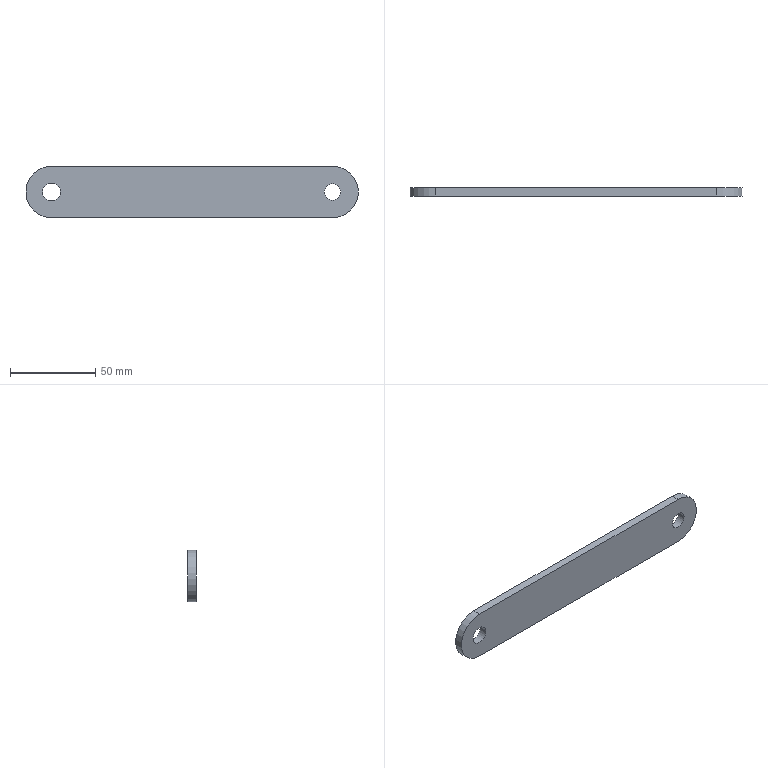Part | NX | features BREP 1 | 1 solid | 10 faces | box 195.262 x 4.763 x 30.163 mm | volume 26365 mm3 | cylinder 6 | plane 4 | commonest cylinder face diameters 9.652 x2 10.414 x2 30.163 x2
STEP:
#1=CARTESIAN_POINT('',(-82.55,0.,15.081));
#2=VERTEX_POINT('',#1);
#3=CARTESIAN_POINT('',(82.55,0.,15.081));
#4=VERTEX_POINT('',#3);
#5=CARTESIAN_POINT('',(-82.55,0.,15.081));
#6=DIRECTION('',(1.,0.,0.));
#7=VECTOR('',#6,1000.);
#8=LINE('',#5,#7);
#9=EDGE_CURVE('',#2,#4,#8,.T.);
#10=ORIENTED_EDGE('',*,*,#9,.T.);
#11=CARTESIAN_POINT('',(82.55,0.,-15.081));
#12=VERTEX_POINT('',#11);
#13=CARTESIAN_POINT('',(82.55,0.,0.));
#14=DIRECTION('',(0.,1.,0.));
#15=DIRECTION('',(0.,0.,1.));
#16=AXIS2_PLACEMENT_3D('',#13,#14,#15);
#17=CIRCLE('',#16,15.081);
#18=EDGE_CURVE('',#4,#12,#17,.T.);
#19=ORIENTED_EDGE('',*,*,#18,.T.);
#20=CARTESIAN_POINT('',(-82.55,0.,-15.081));
#21=VERTEX_POINT('',#20);
#22=CARTESIAN_POINT('',(82.55,0.,-15.081));
#23=DIRECTION('',(-1.,0.,0.));
#24=VECTOR('',#23,1000.);
#25=LINE('',#22,#24);
#26=EDGE_CURVE('',#12,#21,#25,.T.);
#27=ORIENTED_EDGE('',*,*,#26,.T.);
#28=CARTESIAN_POINT('',(-82.55,0.,0.));
#29=DIRECTION('',(0.,1.,0.));
#30=DIRECTION('',(0.,0.,-1.));
#31=AXIS2_PLACEMENT_3D('',#28,#29,#30);
#32=CIRCLE('',#31,15.081);
#33=EDGE_CURVE('',#21,#2,#32,.T.);
#34=ORIENTED_EDGE('',*,*,#33,.T.);
#35=EDGE_LOOP('',(#10,#19,#27,#34));
#36=FACE_BOUND('',#35,.T.);
#37=CARTESIAN_POINT('',(77.724,0.,0.));
#38=VERTEX_POINT('',#37);
#39=CARTESIAN_POINT('',(87.376,0.,0.));
#40=VERTEX_POINT('',#39);
#41=CARTESIAN_POINT('',(82.55,0.,0.));
#42=DIRECTION('',(0.,-1.,0.));
#43=DIRECTION('',(-1.,0.,0.));
#44=AXIS2_PLACEMENT_3D('',#41,#42,#43);
#45=CIRCLE('',#44,4.826);
#46=EDGE_CURVE('',#38,#40,#45,.T.);
#47=ORIENTED_EDGE('',*,*,#46,.T.);
#48=CARTESIAN_POINT('',(82.55,0.,0.));
#49=DIRECTION('',(0.,-1.,0.));
#50=DIRECTION('',(1.,0.,0.));
#51=AXIS2_PLACEMENT_3D('',#48,#49,#50);
#52=CIRCLE('',#51,4.826);
#53=EDGE_CURVE('',#40,#38,#52,.T.);
#54=ORIENTED_EDGE('',*,*,#53,.T.);
#55=EDGE_LOOP('',(#47,#54));
#56=FACE_BOUND('',#55,.T.);
#57=CARTESIAN_POINT('',(-87.757,0.,0.));
#58=VERTEX_POINT('',#57);
#59=CARTESIAN_POINT('',(-77.343,0.,0.));
#60=VERTEX_POINT('',#59);
#61=CARTESIAN_POINT('',(-82.55,0.,0.));
#62=DIRECTION('',(0.,-1.,0.));
#63=DIRECTION('',(-1.,0.,0.));
#64=AXIS2_PLACEMENT_3D('',#61,#62,#63);
#65=CIRCLE('',#64,5.207);
#66=EDGE_CURVE('',#58,#60,#65,.T.);
#67=ORIENTED_EDGE('',*,*,#66,.T.);
#68=CARTESIAN_POINT('',(-82.55,0.,0.));
#69=DIRECTION('',(0.,-1.,0.));
#70=DIRECTION('',(1.,0.,0.));
#71=AXIS2_PLACEMENT_3D('',#68,#69,#70);
#72=CIRCLE('',#71,5.207);
#73=EDGE_CURVE('',#60,#58,#72,.T.);
#74=ORIENTED_EDGE('',*,*,#73,.T.);
#75=EDGE_LOOP('',(#67,#74));
#76=FACE_BOUND('',#75,.T.);
#77=CARTESIAN_POINT('',(0.,0.,0.));
#78=DIRECTION('',(0.,1.,0.));
#79=DIRECTION('',(1.,0.,0.));
#80=AXIS2_PLACEMENT_3D('',#77,#78,#79);
#81=PLANE('',#80);
#82=ADVANCED_FACE('',(#36,#56,#76),#81,.T.);
#83=CARTESIAN_POINT('',(-82.55,-4.763,-15.081));
#84=VERTEX_POINT('',#83);
#85=CARTESIAN_POINT('',(-82.55,0.,-15.081));
#86=DIRECTION('',(0.,-1.,0.));
#87=VECTOR('',#86,1000.);
#88=LINE('',#85,#87);
#89=EDGE_CURVE('',#21,#84,#88,.T.);
#90=ORIENTED_EDGE('',*,*,#89,.T.);
#91=CARTESIAN_POINT('',(-82.55,-4.763,15.081));
#92=VERTEX_POINT('',#91);
#93=CARTESIAN_POINT('',(-82.55,-4.763,0.));
#94=DIRECTION('',(0.,1.,0.));
#95=DIRECTION('',(0.,0.,-1.));
#96=AXIS2_PLACEMENT_3D('',#93,#94,#95);
#97=CIRCLE('',#96,15.081);
#98=EDGE_CURVE('',#84,#92,#97,.T.);
#99=ORIENTED_EDGE('',*,*,#98,.T.);
#100=CARTESIAN_POINT('',(-82.55,0.,15.081));
#101=DIRECTION('',(0.,-1.,0.));
#102=VECTOR('',#101,1000.);
#103=LINE('',#100,#102);
#104=EDGE_CURVE('',#2,#92,#103,.T.);
#105=ORIENTED_EDGE('',*,*,#104,.F.);
#106=ORIENTED_EDGE('',*,*,#33,.F.);
#107=EDGE_LOOP('',(#90,#99,#105,#106));
#108=FACE_BOUND('',#107,.T.);
#109=CARTESIAN_POINT('',(-82.55,-2.381,0.));
#110=DIRECTION('',(0.,1.,0.));
#111=DIRECTION('',(0.,0.,-1.));
#112=AXIS2_PLACEMENT_3D('',#109,#110,#111);
#113=CYLINDRICAL_SURFACE('',#112,15.081);
#114=ADVANCED_FACE('',(#108),#113,.T.);
#115=ORIENTED_EDGE('',*,*,#104,.T.);
#116=CARTESIAN_POINT('',(82.55,-4.763,15.081));
#117=VERTEX_POINT('',#116);
#118=CARTESIAN_POINT('',(-82.55,-4.763,15.081));
#119=DIRECTION('',(1.,0.,0.));
#120=VECTOR('',#119,1000.);
#121=LINE('',#118,#120);
#122=EDGE_CURVE('',#92,#117,#121,.T.);
#123=ORIENTED_EDGE('',*,*,#122,.T.);
#124=CARTESIAN_POINT('',(82.55,0.,15.081));
#125=DIRECTION('',(0.,-1.,0.));
#126=VECTOR('',#125,1000.);
#127=LINE('',#124,#126);
#128=EDGE_CURVE('',#4,#117,#127,.T.);
#129=ORIENTED_EDGE('',*,*,#128,.F.);
#130=ORIENTED_EDGE('',*,*,#9,.F.);
#131=EDGE_LOOP('',(#115,#123,#129,#130));
#132=FACE_BOUND('',#131,.T.);
#133=CARTESIAN_POINT('',(0.,-2.381,15.081));
#134=DIRECTION('',(0.,0.,1.));
#135=DIRECTION('',(1.,0.,0.));
#136=AXIS2_PLACEMENT_3D('',#133,#134,#135);
#137=PLANE('',#136);
#138=ADVANCED_FACE('',(#132),#137,.T.);
#139=ORIENTED_EDGE('',*,*,#128,.T.);
#140=CARTESIAN_POINT('',(82.55,-4.763,-15.081));
#141=VERTEX_POINT('',#140);
#142=CARTESIAN_POINT('',(82.55,-4.763,0.));
#143=DIRECTION('',(0.,1.,0.));
#144=DIRECTION('',(0.,0.,1.));
#145=AXIS2_PLACEMENT_3D('',#142,#143,#144);
#146=CIRCLE('',#145,15.081);
#147=EDGE_CURVE('',#117,#141,#146,.T.);
#148=ORIENTED_EDGE('',*,*,#147,.T.);
#149=CARTESIAN_POINT('',(82.55,0.,-15.081));
#150=DIRECTION('',(0.,-1.,0.));
#151=VECTOR('',#150,1000.);
#152=LINE('',#149,#151);
#153=EDGE_CURVE('',#12,#141,#152,.T.);
#154=ORIENTED_EDGE('',*,*,#153,.F.);
#155=ORIENTED_EDGE('',*,*,#18,.F.);
#156=EDGE_LOOP('',(#139,#148,#154,#155));
#157=FACE_BOUND('',#156,.T.);
#158=CARTESIAN_POINT('',(82.55,-2.381,0.));
#159=DIRECTION('',(0.,1.,0.));
#160=DIRECTION('',(0.,0.,1.));
#161=AXIS2_PLACEMENT_3D('',#158,#159,#160);
#162=CYLINDRICAL_SURFACE('',#161,15.081);
#163=ADVANCED_FACE('',(#157),#162,.T.);
#164=ORIENTED_EDGE('',*,*,#153,.T.);
#165=CARTESIAN_POINT('',(82.55,-4.763,-15.081));
#166=DIRECTION('',(-1.,0.,0.));
#167=VECTOR('',#166,1000.);
#168=LINE('',#165,#167);
#169=EDGE_CURVE('',#141,#84,#168,.T.);
#170=ORIENTED_EDGE('',*,*,#169,.T.);
#171=ORIENTED_EDGE('',*,*,#89,.F.);
#172=ORIENTED_EDGE('',*,*,#26,.F.);
#173=EDGE_LOOP('',(#164,#170,#171,#172));
#174=FACE_BOUND('',#173,.T.);
#175=CARTESIAN_POINT('',(0.,-2.381,-15.081));
#176=DIRECTION('',(0.,0.,-1.));
#177=DIRECTION('',(0.,-1.,0.));
#178=AXIS2_PLACEMENT_3D('',#175,#176,#177);
#179=PLANE('',#178);
#180=ADVANCED_FACE('',(#174),#179,.T.);
#181=ORIENTED_EDGE('',*,*,#169,.F.);
#182=ORIENTED_EDGE('',*,*,#147,.F.);
#183=ORIENTED_EDGE('',*,*,#122,.F.);
#184=ORIENTED_EDGE('',*,*,#98,.F.);
#185=EDGE_LOOP('',(#181,#182,#183,#184));
#186=FACE_BOUND('',#185,.T.);
#187=CARTESIAN_POINT('',(77.724,-4.763,0.));
#188=VERTEX_POINT('',#187);
#189=CARTESIAN_POINT('',(87.376,-4.763,0.));
#190=VERTEX_POINT('',#189);
#191=CARTESIAN_POINT('',(82.55,-4.763,0.));
#192=DIRECTION('',(0.,-1.,0.));
#193=DIRECTION('',(-1.,0.,0.));
#194=AXIS2_PLACEMENT_3D('',#191,#192,#193);
#195=CIRCLE('',#194,4.826);
#196=EDGE_CURVE('',#188,#190,#195,.T.);
#197=ORIENTED_EDGE('',*,*,#196,.F.);
#198=CARTESIAN_POINT('',(82.55,-4.763,0.));
#199=DIRECTION('',(0.,-1.,0.));
#200=DIRECTION('',(1.,0.,0.));
#201=AXIS2_PLACEMENT_3D('',#198,#199,#200);
#202=CIRCLE('',#201,4.826);
#203=EDGE_CURVE('',#190,#188,#202,.T.);
#204=ORIENTED_EDGE('',*,*,#203,.F.);
#205=EDGE_LOOP('',(#197,#204));
#206=FACE_BOUND('',#205,.T.);
#207=CARTESIAN_POINT('',(-87.757,-4.763,0.));
#208=VERTEX_POINT('',#207);
#209=CARTESIAN_POINT('',(-77.343,-4.763,0.));
#210=VERTEX_POINT('',#209);
#211=CARTESIAN_POINT('',(-82.55,-4.763,0.));
#212=DIRECTION('',(0.,-1.,0.));
#213=DIRECTION('',(-1.,0.,0.));
#214=AXIS2_PLACEMENT_3D('',#211,#212,#213);
#215=CIRCLE('',#214,5.207);
#216=EDGE_CURVE('',#208,#210,#215,.T.);
#217=ORIENTED_EDGE('',*,*,#216,.F.);
#218=CARTESIAN_POINT('',(-82.55,-4.763,0.));
#219=DIRECTION('',(0.,-1.,0.));
#220=DIRECTION('',(1.,0.,0.));
#221=AXIS2_PLACEMENT_3D('',#218,#219,#220);
#222=CIRCLE('',#221,5.207);
#223=EDGE_CURVE('',#210,#208,#222,.T.);
#224=ORIENTED_EDGE('',*,*,#223,.F.);
#225=EDGE_LOOP('',(#217,#224));
#226=FACE_BOUND('',#225,.T.);
#227=CARTESIAN_POINT('',(0.,-4.763,0.));
#228=DIRECTION('',(0.,1.,0.));
#229=DIRECTION('',(1.,0.,0.));
#230=AXIS2_PLACEMENT_3D('',#227,#228,#229);
#231=PLANE('',#230);
#232=ADVANCED_FACE('',(#186,#206,#226),#231,.F.);
#233=CARTESIAN_POINT('',(87.376,0.,0.));
#234=DIRECTION('',(0.,-1.,0.));
#235=VECTOR('',#234,1000.);
#236=LINE('',#233,#235);
#237=EDGE_CURVE('',#190,#40,#236,.F.);
#238=ORIENTED_EDGE('',*,*,#237,.F.);
#239=ORIENTED_EDGE('',*,*,#203,.T.);
#240=CARTESIAN_POINT('',(77.724,0.,0.));
#241=DIRECTION('',(0.,-1.,0.));
#242=VECTOR('',#241,1000.);
#243=LINE('',#240,#242);
#244=EDGE_CURVE('',#188,#38,#243,.F.);
#245=ORIENTED_EDGE('',*,*,#244,.T.);
#246=ORIENTED_EDGE('',*,*,#53,.F.);
#247=EDGE_LOOP('',(#238,#239,#245,#246));
#248=FACE_BOUND('',#247,.T.);
#249=CARTESIAN_POINT('',(82.55,0.,0.));
#250=DIRECTION('',(0.,-1.,0.));
#251=DIRECTION('',(1.,0.,0.));
#252=AXIS2_PLACEMENT_3D('',#249,#250,#251);
#253=CYLINDRICAL_SURFACE('',#252,4.826);
#254=ADVANCED_FACE('',(#248),#253,.F.);
#255=ORIENTED_EDGE('',*,*,#244,.F.);
#256=ORIENTED_EDGE('',*,*,#196,.T.);
#257=ORIENTED_EDGE('',*,*,#237,.T.);
#258=ORIENTED_EDGE('',*,*,#46,.F.);
#259=EDGE_LOOP('',(#255,#256,#257,#258));
#260=FACE_BOUND('',#259,.T.);
#261=CARTESIAN_POINT('',(82.55,0.,0.));
#262=DIRECTION('',(0.,-1.,0.));
#263=DIRECTION('',(1.,0.,0.));
#264=AXIS2_PLACEMENT_3D('',#261,#262,#263);
#265=CYLINDRICAL_SURFACE('',#264,4.826);
#266=ADVANCED_FACE('',(#260),#265,.F.);
#267=CARTESIAN_POINT('',(-77.343,0.,0.));
#268=DIRECTION('',(0.,-1.,0.));
#269=VECTOR('',#268,1000.);
#270=LINE('',#267,#269);
#271=EDGE_CURVE('',#210,#60,#270,.F.);
#272=ORIENTED_EDGE('',*,*,#271,.F.);
#273=ORIENTED_EDGE('',*,*,#223,.T.);
#274=CARTESIAN_POINT('',(-87.757,0.,0.));
#275=DIRECTION('',(0.,-1.,0.));
#276=VECTOR('',#275,1000.);
#277=LINE('',#274,#276);
#278=EDGE_CURVE('',#208,#58,#277,.F.);
#279=ORIENTED_EDGE('',*,*,#278,.T.);
#280=ORIENTED_EDGE('',*,*,#73,.F.);
#281=EDGE_LOOP('',(#272,#273,#279,#280));
#282=FACE_BOUND('',#281,.T.);
#283=CARTESIAN_POINT('',(-82.55,0.,0.));
#284=DIRECTION('',(0.,-1.,0.));
#285=DIRECTION('',(1.,0.,0.));
#286=AXIS2_PLACEMENT_3D('',#283,#284,#285);
#287=CYLINDRICAL_SURFACE('',#286,5.207);
#288=ADVANCED_FACE('',(#282),#287,.F.);
#289=ORIENTED_EDGE('',*,*,#278,.F.);
#290=ORIENTED_EDGE('',*,*,#216,.T.);
#291=ORIENTED_EDGE('',*,*,#271,.T.);
#292=ORIENTED_EDGE('',*,*,#66,.F.);
#293=EDGE_LOOP('',(#289,#290,#291,#292));
#294=FACE_BOUND('',#293,.T.);
#295=CARTESIAN_POINT('',(-82.55,0.,0.));
#296=DIRECTION('',(0.,-1.,0.));
#297=DIRECTION('',(1.,0.,0.));
#298=AXIS2_PLACEMENT_3D('',#295,#296,#297);
#299=CYLINDRICAL_SURFACE('',#298,5.207);
#300=ADVANCED_FACE('',(#294),#299,.F.);
#301=CLOSED_SHELL('',(#82,#114,#138,#163,#180,#232,#254,#266,#288,#300));
#302=MANIFOLD_SOLID_BREP('',#301);
#303=(LENGTH_UNIT()NAMED_UNIT(*)SI_UNIT(.MILLI.,.METRE.));
#304=UNCERTAINTY_MEASURE_WITH_UNIT(LENGTH_MEASURE(0.00001),#303,'','');
#305=(NAMED_UNIT(*)PLANE_ANGLE_UNIT()SI_UNIT($,.RADIAN.));
#306=(NAMED_UNIT(*)SI_UNIT($,.STERADIAN.)SOLID_ANGLE_UNIT());
#307=(GEOMETRIC_REPRESENTATION_CONTEXT(3)GLOBAL_UNCERTAINTY_ASSIGNED_CONTEXT((#304))GLOBAL_UNIT_ASSIGNED_CONTEXT((#303,#305,#306))REPRESENTATION_CONTEXT('',''));
#308=ADVANCED_BREP_SHAPE_REPRESENTATION('',(#302),#307);